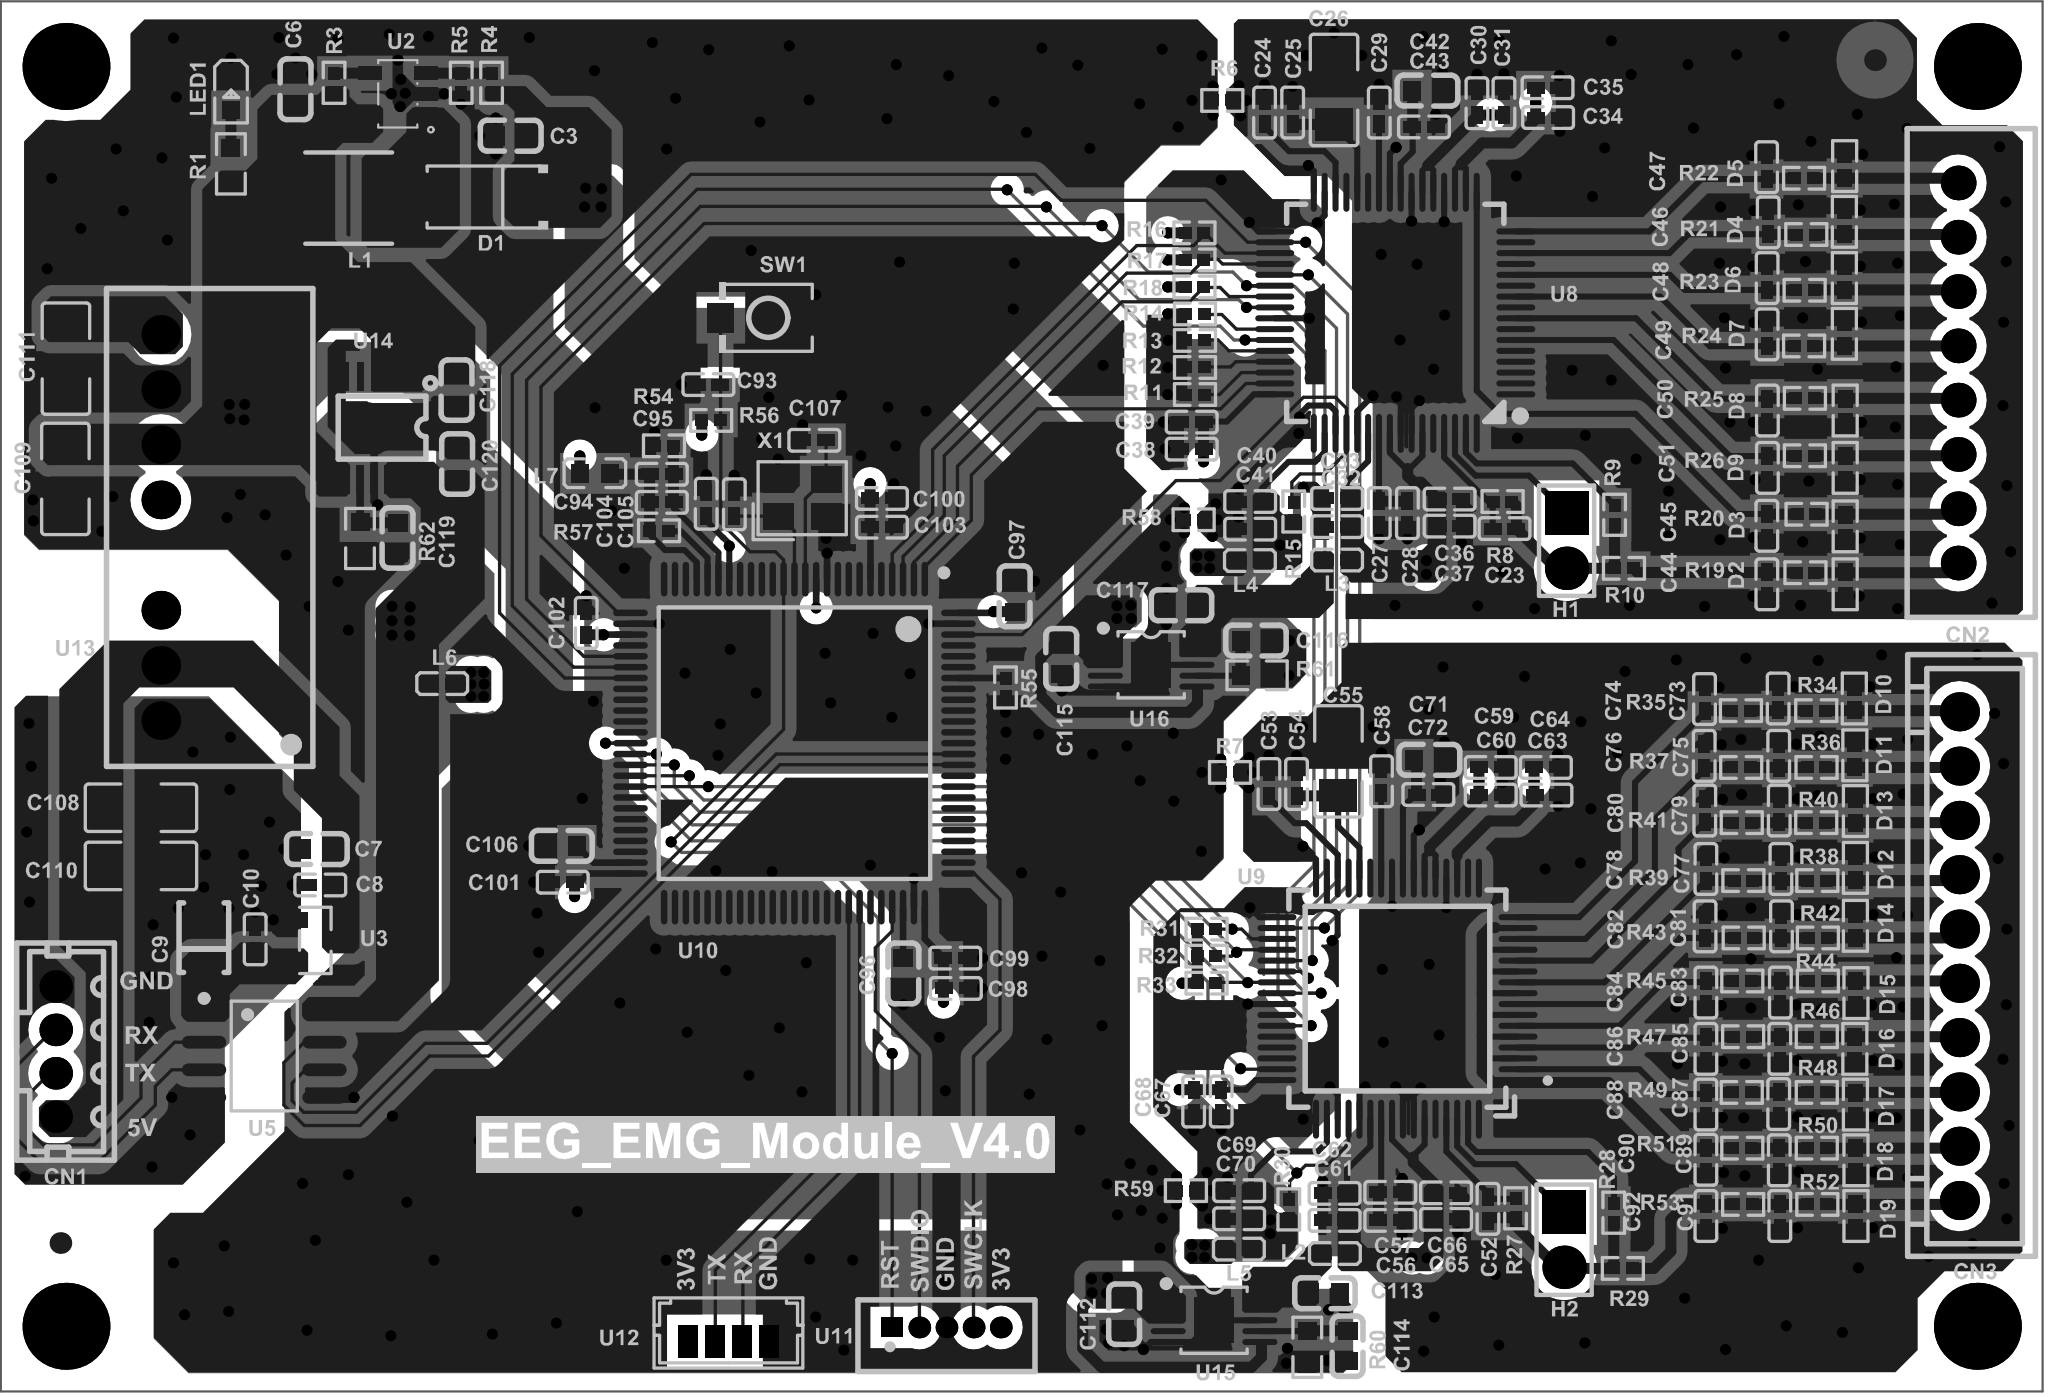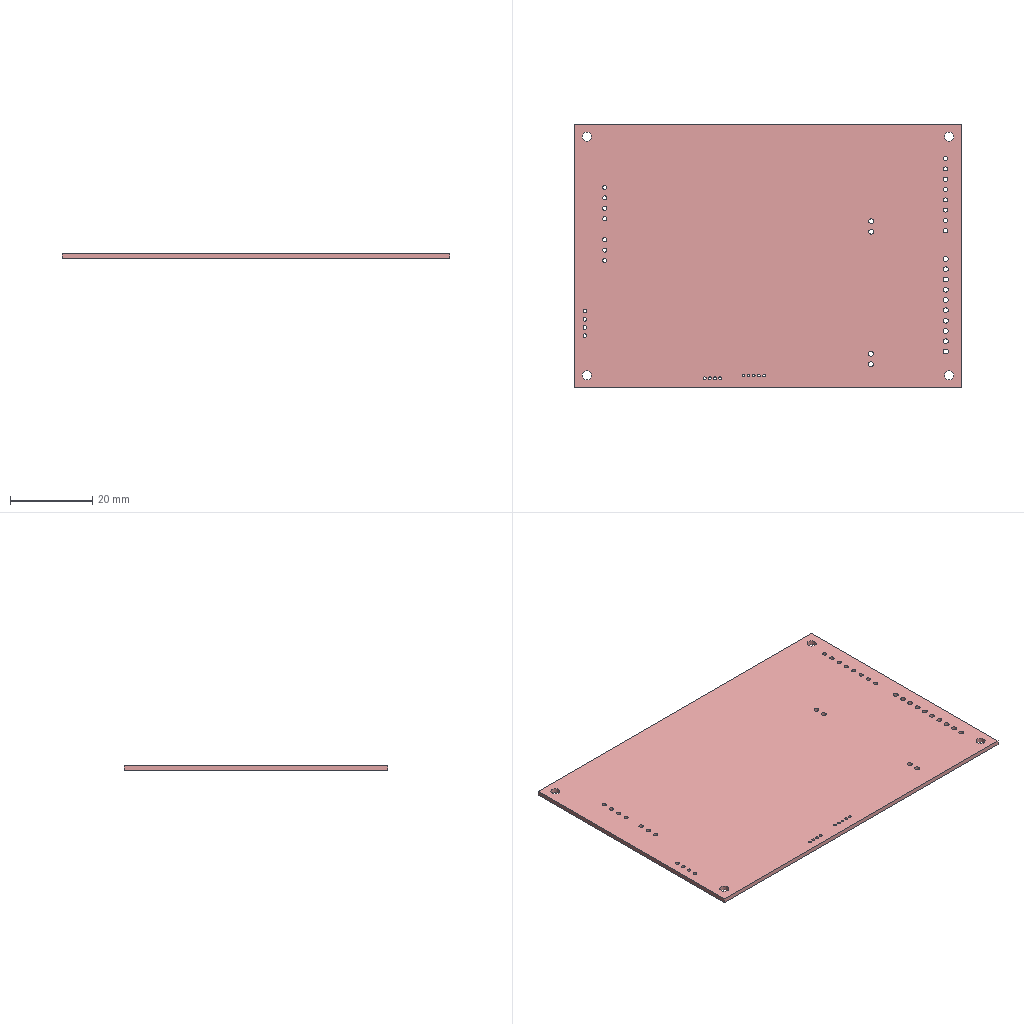Circuit board layout | Altium Designer | box 94 x 64 x 1.1 mm
Part placement:
Designator,Comment,Layer,Footprint,Center-X(mm),Center-Y(mm),Rotation
U16,LT3042EMSE#TRPBF,TopLayer,MSOP-10_L3.0-W3.0-P0.50-LS5.0-BL-EP,52.959,33.452,270
U15,LT3042EMSE#TRPBF,TopLayer,MSOP-10_L3.0-W3.0-P0.50-LS5.0-BL-EP,55.855,3.277,270
U14,LT3045EMSE#TRPBF,TopLayer,MSOP-12_L4.0-W3.0-P0.65-LS4.9-BL-EP,17.514,44.374,180
U13,WRB0505S-3WR2,TopLayer,PWRM-TH_WRA0512S-3WR2,7.366,39.776,90
R62,,TopLayer,R0603,16.535,39.268,90
R61,,TopLayer,R0603,57.836,32.969,360
R60,,TopLayer,R0603,60.147,2.032,90
C120,10uF,TopLayer,C0603,21.006,42.697,270
C119,470nF,TopLayer,C0603,18.263,39.294,90
C118,4.7uF,TopLayer,C0603,20.98,46.101,90
C117,4.7uF,TopLayer,C0603,54.356,36.195,180
C116,470nF,TopLayer,C0603,57.785,34.569,180
C115,4.7uF,TopLayer,C0603,48.819,33.731,90
C114,470nF,TopLayer,C0603,62.001,2.083,90
C113,4.7uF,TopLayer,C0603,60.96,4.521,360
C112,4.7uF,TopLayer,C0603,51.714,3.556,90
C111,22uF,TopLayer,C1206,2.997,47.549,270
C110,47uF,TopLayer,C1206,6.452,24.194,360
C109,100uF,TopLayer,C1206,2.972,42.012,270
C108,100uF,TopLayer,C1206,6.452,26.873,360
R59,,TopLayer,R0402,54.559,9.246,180
R58,,TopLayer,R0402,54.915,40.132,180
X1,8MHz,TopLayer,CRYSTAL-SMD_4P-L3.2-W2.5-BL,36.893,41.123,360
U12,WAFER-MX1.25-4PZZ,TopLayer,CONN-TH_4P-P1.25_WAFER-MX1.25-4PZZ,33.503,2.286,180
U11,WAFER-MX1.25-5PZZ,TopLayer,CONN-TH_5P-P1.25_XUNPU_WAFER-MX1.25-5PZZ,43.536,2.946,360
U10,STM32F407VGT6,TopLayer,LQFP-100_L14.0-W14.0-P0.50-LS16.0-BL,36.537,29.845,180
U9,ADS1298IPAGR,TopLayer,TQFP-64_L10.0-W10.0-P0.50-LS12.0-BL,64.3,18.085,90
U8,ADS1299IPAGR,TopLayer,TQFP-64_L10.0-W10.0-P0.50-LS12.0-TL,64.198,49.657,180
U5,,TopLayer,SOIC-8_L4.9-W3.9-P1.27-LS6.0-BL,12.128,15.443,270
U3,LN6206P332MR-G,TopLayer,SOT-23-3_L2.9-W1.3-P1.90-LS2.4-BR,14.478,20.765,180
U2,MT3540,TopLayer,SOT-23-5_L3.0-W1.7-P0.95-LS2.8-BR,18.275,59.741,360
SW1,TS-1088-AR02016,TopLayer,SW-SMD_L3.9-W3.0-P4.45,35.331,49.428,180
R57,,TopLayer,R0402,30.302,39.624,360
R56,,TopLayer,R0402,32.702,44.704,180
R55,,TopLayer,R0402,46.253,32.41,270
R54,,TopLayer,R0402,30.531,43.536,360
R53,,TopLayer,R0402,80.213,8.611,180
R52,,TopLayer,R0402,83.629,8.611,180
R51,,TopLayer,R0402,80.175,11.201,180
R50,,TopLayer,R0402,83.604,11.201,180
R49,,TopLayer,R0402,80.149,13.767,180
R48,,TopLayer,R0402,83.604,13.767,180
R47,,TopLayer,R0402,80.213,16.332,180
R46,,TopLayer,R0402,83.604,16.332,180
R45,,TopLayer,R0402,80.175,18.898,180
R44,,TopLayer,R0402,83.654,18.898,180
R43,,TopLayer,R0402,80.239,20.879,180
R42,,TopLayer,R0402,83.654,20.879,180
R41,,TopLayer,R0402,80.149,26.187,180
R40,,TopLayer,R0402,83.578,26.187,180
R39,,TopLayer,R0402,80.225,23.52,180
R38,,TopLayer,R0402,83.629,23.52,180
R37,,TopLayer,R0402,80.124,28.727,180
R36,,TopLayer,R0402,83.591,28.727,180
R35,,TopLayer,R0402,80.112,31.344,180
R34,,TopLayer,R0402,83.578,31.344,180
R33,,TopLayer,R0402,55.511,18.796,180
R32,,TopLayer,R0402,55.511,20.041,180
R31,,TopLayer,R0402,55.511,21.285,180
R30,,TopLayer,R0402,59.296,8.382,270
R29,,TopLayer,R0402,74.676,5.664,360
R28,,TopLayer,R0402,74.256,8.23,270
R27,,TopLayer,R0402,69.735,8.433,270
R26,,TopLayer,R0402,83.057,43.078,180
R25,,TopLayer,R0402,83.057,45.72,180
R24,,TopLayer,R0402,83.019,48.133,180
R23,,TopLayer,R0402,83.045,50.698,180
R22,,TopLayer,R0402,83.019,55.855,180
R21,,TopLayer,R0402,83.121,53.264,180
R20,,TopLayer,R0402,83.133,40.386,180
R19,,TopLayer,R0402,83.082,37.694,180
R18,,TopLayer,R0402,54.952,50.851,180
R17,,TopLayer,R0402,54.952,52.095,180
R16,,TopLayer,R0402,54.952,53.34,180
R15,,TopLayer,R0402,59.524,40.513,270
R14,,TopLayer,R0402,54.978,49.606,180
R13,,TopLayer,R0402,54.978,48.387,180
R12,,TopLayer,R0402,54.978,47.142,180
R11,,TopLayer,R0402,54.978,45.898,180
R10,,TopLayer,R0402,74.727,37.897,360
R9,,TopLayer,R0402,74.295,40.361,270
R8,,TopLayer,R0402,69.139,40.97,360
R7,,TopLayer,R0402,56.591,28.499,180
R6,,TopLayer,R0402,56.236,59.436,180
R5,,TopLayer,R0402,21.196,60.249,90
R4,,TopLayer,R0402,22.593,60.249,270
R3,,TopLayer,R0402,15.342,60.249,270
R1,,TopLayer,R0603,10.592,56.515,90
LED1,KT-0603R,TopLayer,LED0603-RD,10.592,59.792,270
L7,GZ1608D601TF,TopLayer,L0603,27.356,42.266,360
L6,BLM15PD121SN1D,TopLayer,L0402,20.32,32.588,360
L5,BLM15PD121SN1D,TopLayer,L0402,56.998,6.553,360
L4,BLM15PD121SN1D,TopLayer,L0402,57.506,38.252,360
L3,BLM15PD121SN1D,TopLayer,L0402,61.519,38.278,360
L2,BLM15PD121SN1D,TopLayer,L0402,61.417,6.35,360
L1,4.7uH,TopLayer,IND-SMD_L4.0-W4.0_FNR40XXS,16.014,54.94,180
H2,PZ254V-11-02P-YL,TopLayer,HDR-TH_2P-P2.54-V-M,71.97,6.985,270
H1,PZ254V-11-02P-YL,TopLayer,HDR-TH_2P-P2.54-V-M,72.085,39.167,270
D19,TPD1E10B06DPYR-TP,TopLayer,X1-DFN1006-2_L1.0-W0.6-BI,85.407,8.077,90
D18,TPD1E10B06DPYR-TP,TopLayer,X1-DFN1006-2_L1.0-W0.6-BI,85.407,10.643,90
D17,TPD1E10B06DPYR-TP,TopLayer,X1-DFN1006-2_L1.0-W0.6-BI,85.382,13.208,90
D16,TPD1E10B06DPYR-TP,TopLayer,X1-DFN1006-2_L1.0-W0.6-BI,85.356,15.773,90
D15,TPD1E10B06DPYR-TP,TopLayer,X1-DFN1006-2_L1.0-W0.6-BI,85.407,18.339,90
D14,TPD1E10B06DPYR-TP,TopLayer,X1-DFN1006-2_L1.0-W0.6-BI,85.382,21.438,270
D13,TPD1E10B06DPYR-TP,TopLayer,X1-DFN1006-2_L1.0-W0.6-BI,85.382,26.721,270
D12,TPD1E10B06DPYR-TP,TopLayer,X1-DFN1006-2_L1.0-W0.6-BI,85.382,24.105,270
D11,TPD1E10B06DPYR-TP,TopLayer,X1-DFN1006-2_L1.0-W0.6-BI,85.356,29.286,270
D10,TPD1E10B06DPYR-TP,TopLayer,X1-DFN1006-2_L1.0-W0.6-BI,85.331,31.902,270
D9,TPD1E10B06DPYR-TP,TopLayer,X1-DFN1006-2_L1.0-W0.6-BI,84.911,42.52,90
D8,TPD1E10B06DPYR-TP,TopLayer,X1-DFN1006-2_L1.0-W0.6-BI,84.911,45.161,90
D7,TPD1E10B06DPYR-TP,TopLayer,X1-DFN1006-2_L1.0-W0.6-BI,84.874,48.692,270
D6,TPD1E10B06DPYR-TP,TopLayer,X1-DFN1006-2_L1.0-W0.6-BI,84.874,51.257,270
D5,TPD1E10B06DPYR-TP,TopLayer,X1-DFN1006-2_L1.0-W0.6-BI,84.887,56.413,270
D4,TPD1E10B06DPYR-TP,TopLayer,X1-DFN1006-2_L1.0-W0.6-BI,84.874,53.848,270
D3,TPD1E10B06DPYR-TP,TopLayer,X1-DFN1006-2_L1.0-W0.6-BI,84.911,39.827,90
D2,TPD1E10B06DPYR-TP,TopLayer,X1-DFN1006-2_L1.0-W0.6-BI,84.911,37.16,90
D1,B340LA-13-F,TopLayer,SMA_L4.3-W2.6-LS5.2-RD,22.225,54.991,180
CN3,A2501WV-10P,TopLayer,CONN-TH_A2501WV-10P,90.17,20.041,270
CN2,WF-1A254A8P,TopLayer,CONN-TH_WF-1A254A8P,90.114,46.888,270
CN1,A2001WV-4P,TopLayer,CONN-TH_A2001WV-4P,2.527,15.646,270
C107,12pF,TopLayer,C0402,37.452,43.79,360
C106,2.2uF,TopLayer,C0603,25.819,25.121,180
C105,12pF,TopLayer,C0402,33.769,40.843,270
C104,100nF,TopLayer,C0402,32.473,40.869,270
C103,100nF,TopLayer,C0402,40.564,39.79,180
C102,100nF,TopLayer,C0402,26.949,35.382,270
C101,100nF,TopLayer,C0402,25.869,23.444,360
C100,100nF,TopLayer,C0402,40.564,41.11,180
C99,100nF,TopLayer,C0402,43.942,19.951,180
C98,100nF,TopLayer,C0402,43.967,18.554,180
C97,10uF,TopLayer,C0603,46.672,36.601,270
C96,2.2uF,TopLayer,C0603,41.554,19.253,90
C95,1uF,TopLayer,C0402,30.429,42.228,180
C94,100nF,TopLayer,C0402,30.429,40.933,180
C93,100nF,TopLayer,C0402,32.575,46.355,360
C92,47pF,TopLayer,C0402,78.498,8.077,90
C91,47pF,TopLayer,C0402,81.902,8.077,90
C90,47pF,TopLayer,C0402,78.498,10.668,90
C89,47pF,TopLayer,C0402,81.876,10.643,90
C88,47pF,TopLayer,C0402,78.498,13.208,90
C87,47pF,TopLayer,C0402,81.851,13.233,90
C86,47pF,TopLayer,C0402,78.498,15.773,90
C85,47pF,TopLayer,C0402,81.902,15.773,90
C84,47pF,TopLayer,C0402,78.498,18.364,90
C83,47pF,TopLayer,C0402,81.927,18.364,90
C82,47pF,TopLayer,C0402,78.461,21.412,270
C81,47pF,TopLayer,C0402,81.978,21.412,270
C80,47pF,TopLayer,C0402,78.447,26.746,270
C79,47pF,TopLayer,C0402,81.876,26.746,270
C78,47pF,TopLayer,C0402,78.498,24.054,270
C77,47pF,TopLayer,C0402,81.953,24.054,270
C76,47pF,TopLayer,C0402,78.422,29.261,270
C75,47pF,TopLayer,C0402,81.851,29.261,270
C74,47pF,TopLayer,C0402,78.435,31.877,270
C73,47pF,TopLayer,C0402,81.826,31.902,270
C72,100nF,TopLayer,C0402,65.722,27.483,180
C71,10uF,TopLayer,C0603,65.761,29.083,180
C70,100nF,TopLayer,C0402,57.01,7.95,360
C69,1uF,TopLayer,C0402,57.01,9.246,360
C68,100nF,TopLayer,C0402,54.915,13.348,270
C67,1uF,TopLayer,C0402,56.185,13.348,270
C66,100nF,TopLayer,C0402,66.535,9.144,180
C65,1uF,TopLayer,C0402,66.535,7.925,180
C64,100nF,TopLayer,C0402,71.132,28.727,180
C63,1uF,TopLayer,C0402,71.158,27.457,180
C62,100nF,TopLayer,C0402,61.404,9.119,180
C61,1uF,TopLayer,C0402,61.404,7.874,180
C60,100nF,TopLayer,C0402,68.592,27.457,180
C59,1uF,TopLayer,C0402,68.592,28.727,180
C58,1uF,TopLayer,C0402,63.563,28.092,90
C57,100nF,TopLayer,C0402,63.969,9.169,180
C56,1uF,TopLayer,C0402,63.969,7.874,180
C55,22uF,TopLayer,C1206,61.582,29.007,270
C54,1uF,TopLayer,C0402,59.651,27.965,270
C53,1uF,TopLayer,C0402,58.381,27.965,90
C52,1.5nF,TopLayer,C0402,68.465,8.407,90
C51,4.7nF,TopLayer,C0402,81.33,42.52,90
C50,4.7nF,TopLayer,C0402,81.33,45.161,90
C49,4.7nF,TopLayer,C0402,81.318,48.666,270
C48,4.7nF,TopLayer,C0402,81.318,51.257,270
C47,4.7nF,TopLayer,C0402,81.292,56.363,270
C46,4.7nF,TopLayer,C0402,81.368,53.823,270
C45,4.7nF,TopLayer,C0402,81.304,39.853,90
C44,4.7nF,TopLayer,C0402,81.304,37.16,90
C43,100nF,TopLayer,C0402,65.519,58.217,180
C42,10uF,TopLayer,C0603,65.671,59.893,180
C41,100nF,TopLayer,C0402,57.518,39.7,360
C40,1uF,TopLayer,C0402,57.518,40.97,360
C39,100nF,TopLayer,C0402,54.825,44.628,180
C38,1uF,TopLayer,C0402,54.825,43.383,180
C37,100nF,TopLayer,C0402,66.7,39.839,180
C36,1uF,TopLayer,C0402,66.7,41.084,180
C35,100nF,TopLayer,C0402,71.208,60.02,180
C34,1uF,TopLayer,C0402,71.234,58.649,180
C33,100nF,TopLayer,C0402,61.519,41.11,180
C32,1uF,TopLayer,C0402,61.519,39.815,180
C31,100nF,TopLayer,C0402,69.202,59.309,270
C30,1uF,TopLayer,C0402,67.957,59.309,270
C29,1uF,TopLayer,C0402,63.461,58.877,90
C28,100nF,TopLayer,C0402,64.757,40.437,90
C27,1uF,TopLayer,C0402,63.461,40.437,90
C26,100uF,TopLayer,C1206,61.379,59.919,270
C25,1uF,TopLayer,C0402,59.474,58.877,270
C24,1uF,TopLayer,C0402,58.178,58.877,90
C23,10nF,TopLayer,C0402,69.227,39.726,180
C10,1uF,TopLayer,C0402,11.709,20.816,270
C9,22uF,TopLayer,CAP-SMD_L3.2-W1.6,9.347,20.892,90
C8,1uF,TopLayer,C0402,14.707,23.317,360
C7,10uF,TopLayer,C0603,14.554,24.968,360
C6,10uF,TopLayer,C0603,13.564,59.944,270
C3,10uF,TopLayer,C0603,23.482,57.81,360